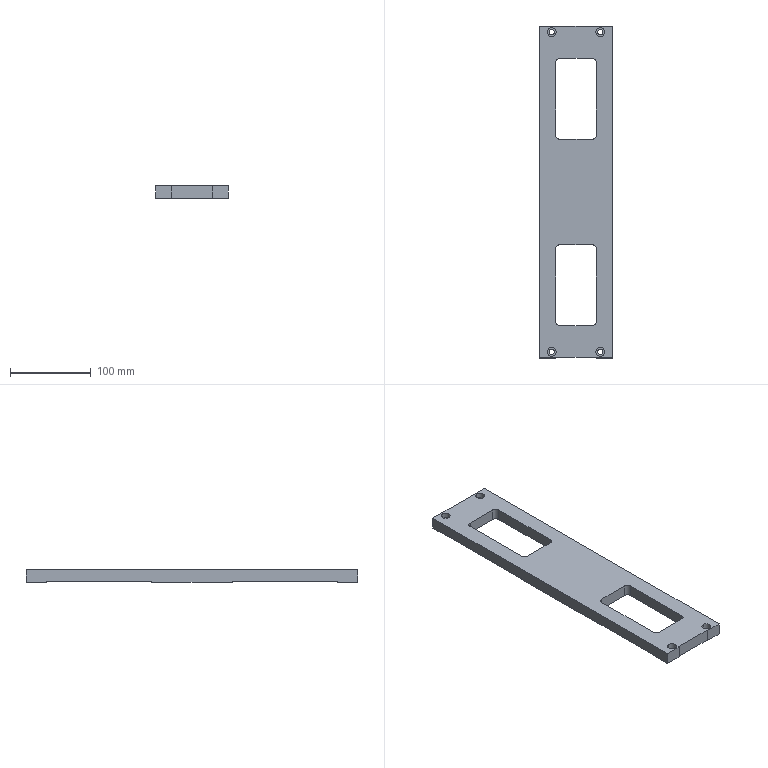Part | 1 solid | 94 faces | box 90 x 410 x 15 mm | volume 391776 mm3 | cylinder 44 | plane 30 | cone 20 | commonest cylinder face diameters 3.3 x8 4 x8 6.6 x8 10 x8 11 x8 6 x4